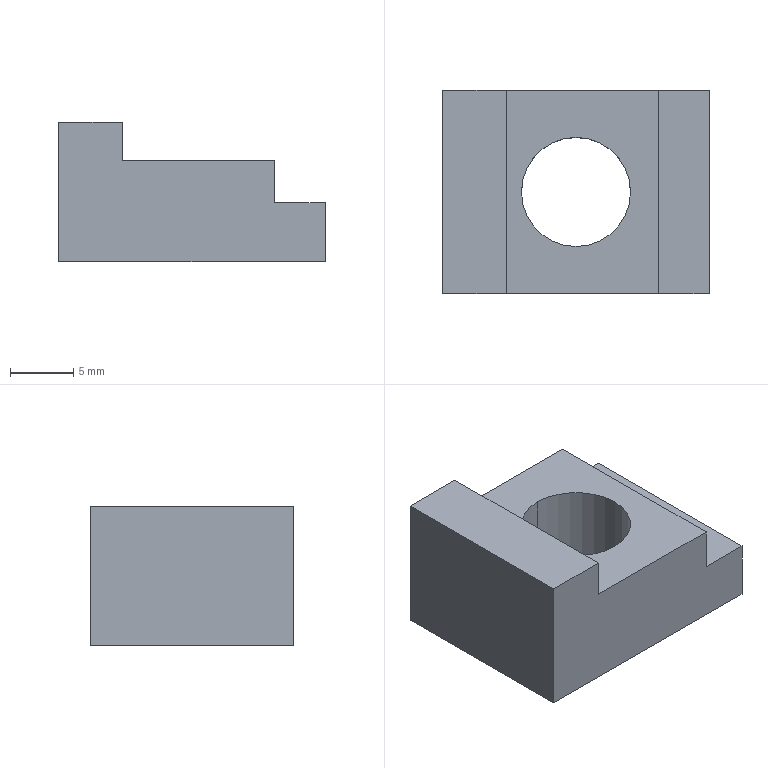Part | STEP file | 1_id1418_x_t | 1 solid | 12 faces | box 21 x 16 x 11 mm | volume 2249 mm3 | plane 10 | cylinder 2 | commonest cylinder face diameters 8.6 x2
STEP:
#1=CARTESIAN_POINT('',(0.,0.,0.));
#2=DIRECTION('',(0.,0.,1.));
#3=DIRECTION('',(1.,0.,0.));
#4=AXIS2_PLACEMENT_3D('',#1,#2,#3);
#5=CARTESIAN_POINT('',(17.925,355.5,90.11));
#6=VERTEX_POINT('',#5);
#7=CARTESIAN_POINT('',(17.925,355.5,79.11));
#8=VERTEX_POINT('',#7);
#9=CARTESIAN_POINT('',(17.925,355.5,90.11));
#10=DIRECTION('',(0.,0.,-1.));
#11=VECTOR('',#10,1.);
#12=LINE('',#9,#11);
#13=CARTESIAN_POINT('',(17.925,355.5,79.11));
#14=DIRECTION('',(1.,0.,0.));
#15=DIRECTION('',(0.,-1.,0.));
#16=AXIS2_PLACEMENT_3D('',#13,#14,#15);
#17=PLANE('',#16);
#18=CARTESIAN_POINT('',(0.,-11.));
#19=DIRECTION('',(0.,1.));
#20=VECTOR('',#19,1.);
#21=LINE('',#18,#20);
#22=(GEOMETRIC_REPRESENTATION_CONTEXT(2)PARAMETRIC_REPRESENTATION_CONTEXT()REPRESENTATION_CONTEXT('',''));
#23=DEFINITIONAL_REPRESENTATION('',(#21),#22);
#24=PCURVE('',#17,#23);
#25=CARTESIAN_POINT('',(38.925,355.5,79.11));
#26=DIRECTION('',(0.,-1.,0.));
#27=DIRECTION('',(0.,0.,1.));
#28=AXIS2_PLACEMENT_3D('',#25,#26,#27);
#29=PLANE('',#28);
#30=CARTESIAN_POINT('',(11.,21.));
#31=DIRECTION('',(-1.,0.));
#32=VECTOR('',#31,1.);
#33=LINE('',#30,#32);
#34=(GEOMETRIC_REPRESENTATION_CONTEXT(2)PARAMETRIC_REPRESENTATION_CONTEXT()REPRESENTATION_CONTEXT('',''));
#35=DEFINITIONAL_REPRESENTATION('',(#33),#34);
#36=PCURVE('',#29,#35);
#37=SURFACE_CURVE('',#12,(#24,#36),.PCURVE_S1.);
#38=EDGE_CURVE('',#6,#8,#37,.T.);
#39=ORIENTED_EDGE('',*,*,#38,.T.);
#40=CARTESIAN_POINT('',(17.925,339.5,79.11));
#41=VERTEX_POINT('',#40);
#42=CARTESIAN_POINT('',(17.925,339.5,79.11));
#43=DIRECTION('',(0.,1.,0.));
#44=VECTOR('',#43,1.);
#45=LINE('',#42,#44);
#46=CARTESIAN_POINT('',(16.,0.));
#47=DIRECTION('',(-1.,0.));
#48=VECTOR('',#47,1.);
#49=LINE('',#46,#48);
#50=(GEOMETRIC_REPRESENTATION_CONTEXT(2)PARAMETRIC_REPRESENTATION_CONTEXT()REPRESENTATION_CONTEXT('',''));
#51=DEFINITIONAL_REPRESENTATION('',(#49),#50);
#52=PCURVE('',#17,#51);
#53=CARTESIAN_POINT('',(38.925,339.5,79.11));
#54=DIRECTION('',(0.,0.,-1.));
#55=DIRECTION('',(-0.5,0.866,0.));
#56=AXIS2_PLACEMENT_3D('',#53,#54,#55);
#57=PLANE('',#56);
#58=CARTESIAN_POINT('',(10.5,-18.187));
#59=DIRECTION('',(0.866,0.5));
#60=VECTOR('',#59,1.);
#61=LINE('',#58,#60);
#62=(GEOMETRIC_REPRESENTATION_CONTEXT(2)PARAMETRIC_REPRESENTATION_CONTEXT()REPRESENTATION_CONTEXT('',''));
#63=DEFINITIONAL_REPRESENTATION('',(#61),#62);
#64=PCURVE('',#57,#63);
#65=SURFACE_CURVE('',#45,(#52,#64),.PCURVE_S1.);
#66=EDGE_CURVE('',#41,#8,#65,.T.);
#67=ORIENTED_EDGE('',*,*,#66,.F.);
#68=CARTESIAN_POINT('',(17.925,339.5,90.11));
#69=VERTEX_POINT('',#68);
#70=CARTESIAN_POINT('',(17.925,339.5,90.11));
#71=DIRECTION('',(0.,0.,-1.));
#72=VECTOR('',#71,1.);
#73=LINE('',#70,#72);
#74=CARTESIAN_POINT('',(16.,-11.));
#75=DIRECTION('',(0.,1.));
#76=VECTOR('',#75,1.);
#77=LINE('',#74,#76);
#78=(GEOMETRIC_REPRESENTATION_CONTEXT(2)PARAMETRIC_REPRESENTATION_CONTEXT()REPRESENTATION_CONTEXT('',''));
#79=DEFINITIONAL_REPRESENTATION('',(#77),#78);
#80=PCURVE('',#17,#79);
#81=CARTESIAN_POINT('',(17.925,339.5,79.11));
#82=DIRECTION('',(0.,1.,0.));
#83=DIRECTION('',(0.,0.,-1.));
#84=AXIS2_PLACEMENT_3D('',#81,#82,#83);
#85=PLANE('',#84);
#86=CARTESIAN_POINT('',(-11.,0.));
#87=DIRECTION('',(1.,0.));
#88=VECTOR('',#87,1.);
#89=LINE('',#86,#88);
#90=(GEOMETRIC_REPRESENTATION_CONTEXT(2)PARAMETRIC_REPRESENTATION_CONTEXT()REPRESENTATION_CONTEXT('',''));
#91=DEFINITIONAL_REPRESENTATION('',(#89),#90);
#92=PCURVE('',#85,#91);
#93=SURFACE_CURVE('',#73,(#80,#92),.PCURVE_S1.);
#94=EDGE_CURVE('',#69,#41,#93,.T.);
#95=ORIENTED_EDGE('',*,*,#94,.F.);
#96=CARTESIAN_POINT('',(17.925,355.5,90.11));
#97=DIRECTION('',(0.,-1.,0.));
#98=VECTOR('',#97,1.);
#99=LINE('',#96,#98);
#100=CARTESIAN_POINT('',(0.,-11.));
#101=DIRECTION('',(1.,0.));
#102=VECTOR('',#101,1.);
#103=LINE('',#100,#102);
#104=(GEOMETRIC_REPRESENTATION_CONTEXT(2)PARAMETRIC_REPRESENTATION_CONTEXT()REPRESENTATION_CONTEXT('',''));
#105=DEFINITIONAL_REPRESENTATION('',(#103),#104);
#106=PCURVE('',#17,#105);
#107=CARTESIAN_POINT('',(22.925,355.5,90.11));
#108=DIRECTION('',(0.,0.,1.));
#109=DIRECTION('',(0.866,0.5,0.));
#110=AXIS2_PLACEMENT_3D('',#107,#108,#109);
#111=PLANE('',#110);
#112=CARTESIAN_POINT('',(-4.33,2.5));
#113=DIRECTION('',(-0.5,-0.866));
#114=VECTOR('',#113,1.);
#115=LINE('',#112,#114);
#116=(GEOMETRIC_REPRESENTATION_CONTEXT(2)PARAMETRIC_REPRESENTATION_CONTEXT()REPRESENTATION_CONTEXT('',''));
#117=DEFINITIONAL_REPRESENTATION('',(#115),#116);
#118=PCURVE('',#111,#117);
#119=SURFACE_CURVE('',#99,(#106,#118),.PCURVE_S1.);
#120=EDGE_CURVE('',#6,#69,#119,.T.);
#121=ORIENTED_EDGE('',*,*,#120,.F.);
#122=EDGE_LOOP('',(#39,#67,#95,#121));
#123=FACE_BOUND('',#122,.T.);
#124=ADVANCED_FACE('',(#123),#17,.F.);
#125=ORIENTED_EDGE('',*,*,#120,.T.);
#126=CARTESIAN_POINT('',(22.925,339.5,90.11));
#127=VERTEX_POINT('',#126);
#128=CARTESIAN_POINT('',(17.925,339.5,90.11));
#129=DIRECTION('',(1.,0.,0.));
#130=VECTOR('',#129,1.);
#131=LINE('',#128,#130);
#132=CARTESIAN_POINT('',(-12.33,-11.356));
#133=DIRECTION('',(0.866,-0.5));
#134=VECTOR('',#133,1.);
#135=LINE('',#132,#134);
#136=(GEOMETRIC_REPRESENTATION_CONTEXT(2)PARAMETRIC_REPRESENTATION_CONTEXT()REPRESENTATION_CONTEXT('',''));
#137=DEFINITIONAL_REPRESENTATION('',(#135),#136);
#138=PCURVE('',#111,#137);
#139=CARTESIAN_POINT('',(-11.,0.));
#140=DIRECTION('',(0.,-1.));
#141=VECTOR('',#140,1.);
#142=LINE('',#139,#141);
#143=(GEOMETRIC_REPRESENTATION_CONTEXT(2)PARAMETRIC_REPRESENTATION_CONTEXT()REPRESENTATION_CONTEXT('',''));
#144=DEFINITIONAL_REPRESENTATION('',(#142),#143);
#145=PCURVE('',#85,#144);
#146=SURFACE_CURVE('',#131,(#138,#145),.PCURVE_S1.);
#147=EDGE_CURVE('',#69,#127,#146,.T.);
#148=ORIENTED_EDGE('',*,*,#147,.T.);
#149=CARTESIAN_POINT('',(22.925,355.5,90.11));
#150=VERTEX_POINT('',#149);
#151=CARTESIAN_POINT('',(22.925,339.5,90.11));
#152=DIRECTION('',(0.,1.,0.));
#153=VECTOR('',#152,1.);
#154=LINE('',#151,#153);
#155=CARTESIAN_POINT('',(-8.,-13.856));
#156=DIRECTION('',(0.5,0.866));
#157=VECTOR('',#156,1.);
#158=LINE('',#155,#157);
#159=(GEOMETRIC_REPRESENTATION_CONTEXT(2)PARAMETRIC_REPRESENTATION_CONTEXT()REPRESENTATION_CONTEXT('',''));
#160=DEFINITIONAL_REPRESENTATION('',(#158),#159);
#161=PCURVE('',#111,#160);
#162=CARTESIAN_POINT('',(22.925,355.5,90.11));
#163=DIRECTION('',(-1.,0.,0.));
#164=DIRECTION('',(0.,0.,1.));
#165=AXIS2_PLACEMENT_3D('',#162,#163,#164);
#166=PLANE('',#165);
#167=CARTESIAN_POINT('',(0.,-16.));
#168=DIRECTION('',(0.,1.));
#169=VECTOR('',#168,1.);
#170=LINE('',#167,#169);
#171=(GEOMETRIC_REPRESENTATION_CONTEXT(2)PARAMETRIC_REPRESENTATION_CONTEXT()REPRESENTATION_CONTEXT('',''));
#172=DEFINITIONAL_REPRESENTATION('',(#170),#171);
#173=PCURVE('',#166,#172);
#174=SURFACE_CURVE('',#154,(#161,#173),.PCURVE_S1.);
#175=EDGE_CURVE('',#127,#150,#174,.T.);
#176=ORIENTED_EDGE('',*,*,#175,.T.);
#177=CARTESIAN_POINT('',(22.925,355.5,90.11));
#178=DIRECTION('',(-1.,0.,0.));
#179=VECTOR('',#178,1.);
#180=LINE('',#177,#179);
#181=CARTESIAN_POINT('',(0.,0.));
#182=DIRECTION('',(-0.866,0.5));
#183=VECTOR('',#182,1.);
#184=LINE('',#181,#183);
#185=(GEOMETRIC_REPRESENTATION_CONTEXT(2)PARAMETRIC_REPRESENTATION_CONTEXT()REPRESENTATION_CONTEXT('',''));
#186=DEFINITIONAL_REPRESENTATION('',(#184),#185);
#187=PCURVE('',#111,#186);
#188=CARTESIAN_POINT('',(11.,16.));
#189=DIRECTION('',(0.,1.));
#190=VECTOR('',#189,1.);
#191=LINE('',#188,#190);
#192=(GEOMETRIC_REPRESENTATION_CONTEXT(2)PARAMETRIC_REPRESENTATION_CONTEXT()REPRESENTATION_CONTEXT('',''));
#193=DEFINITIONAL_REPRESENTATION('',(#191),#192);
#194=PCURVE('',#29,#193);
#195=SURFACE_CURVE('',#180,(#187,#194),.PCURVE_S1.);
#196=EDGE_CURVE('',#150,#6,#195,.T.);
#197=ORIENTED_EDGE('',*,*,#196,.T.);
#198=EDGE_LOOP('',(#125,#148,#176,#197));
#199=FACE_BOUND('',#198,.T.);
#200=ADVANCED_FACE('',(#199),#111,.T.);
#201=CARTESIAN_POINT('',(34.925,355.5,83.76));
#202=VERTEX_POINT('',#201);
#203=CARTESIAN_POINT('',(34.925,355.5,87.11));
#204=VERTEX_POINT('',#203);
#205=CARTESIAN_POINT('',(34.925,355.5,83.76));
#206=DIRECTION('',(0.,0.,1.));
#207=VECTOR('',#206,1.);
#208=LINE('',#205,#207);
#209=CARTESIAN_POINT('',(4.65,4.));
#210=DIRECTION('',(1.,0.));
#211=VECTOR('',#210,1.);
#212=LINE('',#209,#211);
#213=(GEOMETRIC_REPRESENTATION_CONTEXT(2)PARAMETRIC_REPRESENTATION_CONTEXT()REPRESENTATION_CONTEXT('',''));
#214=DEFINITIONAL_REPRESENTATION('',(#212),#213);
#215=PCURVE('',#29,#214);
#216=CARTESIAN_POINT('',(34.925,355.5,87.11));
#217=DIRECTION('',(-1.,0.,0.));
#218=DIRECTION('',(0.,0.,1.));
#219=AXIS2_PLACEMENT_3D('',#216,#217,#218);
#220=PLANE('',#219);
#221=CARTESIAN_POINT('',(-3.35,0.));
#222=DIRECTION('',(1.,0.));
#223=VECTOR('',#222,1.);
#224=LINE('',#221,#223);
#225=(GEOMETRIC_REPRESENTATION_CONTEXT(2)PARAMETRIC_REPRESENTATION_CONTEXT()REPRESENTATION_CONTEXT('',''));
#226=DEFINITIONAL_REPRESENTATION('',(#224),#225);
#227=PCURVE('',#220,#226);
#228=SURFACE_CURVE('',#208,(#215,#227),.PCURVE_S1.);
#229=EDGE_CURVE('',#202,#204,#228,.T.);
#230=ORIENTED_EDGE('',*,*,#229,.F.);
#231=CARTESIAN_POINT('',(38.925,355.5,83.76));
#232=VERTEX_POINT('',#231);
#233=CARTESIAN_POINT('',(38.925,355.5,83.76));
#234=DIRECTION('',(-1.,0.,0.));
#235=VECTOR('',#234,1.);
#236=LINE('',#233,#235);
#237=CARTESIAN_POINT('',(4.65,0.));
#238=DIRECTION('',(0.,1.));
#239=VECTOR('',#238,1.);
#240=LINE('',#237,#239);
#241=(GEOMETRIC_REPRESENTATION_CONTEXT(2)PARAMETRIC_REPRESENTATION_CONTEXT()REPRESENTATION_CONTEXT('',''));
#242=DEFINITIONAL_REPRESENTATION('',(#240),#241);
#243=PCURVE('',#29,#242);
#244=CARTESIAN_POINT('',(38.925,339.5,83.76));
#245=DIRECTION('',(0.,0.,-1.));
#246=DIRECTION('',(-0.5,0.866,0.));
#247=AXIS2_PLACEMENT_3D('',#244,#245,#246);
#248=PLANE('',#247);
#249=CARTESIAN_POINT('',(13.856,8.));
#250=DIRECTION('',(0.5,-0.866));
#251=VECTOR('',#250,1.);
#252=LINE('',#249,#251);
#253=(GEOMETRIC_REPRESENTATION_CONTEXT(2)PARAMETRIC_REPRESENTATION_CONTEXT()REPRESENTATION_CONTEXT('',''));
#254=DEFINITIONAL_REPRESENTATION('',(#252),#253);
#255=PCURVE('',#248,#254);
#256=SURFACE_CURVE('',#236,(#243,#255),.PCURVE_S1.);
#257=EDGE_CURVE('',#232,#202,#256,.T.);
#258=ORIENTED_EDGE('',*,*,#257,.F.);
#259=CARTESIAN_POINT('',(38.925,355.5,79.11));
#260=VERTEX_POINT('',#259);
#261=CARTESIAN_POINT('',(38.925,355.5,83.76));
#262=DIRECTION('',(0.,0.,-1.));
#263=VECTOR('',#262,1.);
#264=LINE('',#261,#263);
#265=CARTESIAN_POINT('',(4.65,0.));
#266=DIRECTION('',(-1.,0.));
#267=VECTOR('',#266,1.);
#268=LINE('',#265,#267);
#269=(GEOMETRIC_REPRESENTATION_CONTEXT(2)PARAMETRIC_REPRESENTATION_CONTEXT()REPRESENTATION_CONTEXT('',''));
#270=DEFINITIONAL_REPRESENTATION('',(#268),#269);
#271=PCURVE('',#29,#270);
#272=CARTESIAN_POINT('',(38.925,339.5,79.11));
#273=DIRECTION('',(-1.,0.,0.));
#274=DIRECTION('',(0.,0.,1.));
#275=AXIS2_PLACEMENT_3D('',#272,#273,#274);
#276=PLANE('',#275);
#277=CARTESIAN_POINT('',(4.65,16.));
#278=DIRECTION('',(-1.,0.));
#279=VECTOR('',#278,1.);
#280=LINE('',#277,#279);
#281=(GEOMETRIC_REPRESENTATION_CONTEXT(2)PARAMETRIC_REPRESENTATION_CONTEXT()REPRESENTATION_CONTEXT('',''));
#282=DEFINITIONAL_REPRESENTATION('',(#280),#281);
#283=PCURVE('',#276,#282);
#284=SURFACE_CURVE('',#264,(#271,#283),.PCURVE_S1.);
#285=EDGE_CURVE('',#232,#260,#284,.T.);
#286=ORIENTED_EDGE('',*,*,#285,.T.);
#287=CARTESIAN_POINT('',(17.925,355.5,79.11));
#288=DIRECTION('',(1.,0.,0.));
#289=VECTOR('',#288,1.);
#290=LINE('',#287,#289);
#291=CARTESIAN_POINT('',(0.,21.));
#292=DIRECTION('',(0.,-1.));
#293=VECTOR('',#292,1.);
#294=LINE('',#291,#293);
#295=(GEOMETRIC_REPRESENTATION_CONTEXT(2)PARAMETRIC_REPRESENTATION_CONTEXT()REPRESENTATION_CONTEXT('',''));
#296=DEFINITIONAL_REPRESENTATION('',(#294),#295);
#297=PCURVE('',#29,#296);
#298=CARTESIAN_POINT('',(24.356,-10.187));
#299=DIRECTION('',(-0.5,0.866));
#300=VECTOR('',#299,1.);
#301=LINE('',#298,#300);
#302=(GEOMETRIC_REPRESENTATION_CONTEXT(2)PARAMETRIC_REPRESENTATION_CONTEXT()REPRESENTATION_CONTEXT('',''));
#303=DEFINITIONAL_REPRESENTATION('',(#301),#302);
#304=PCURVE('',#57,#303);
#305=SURFACE_CURVE('',#290,(#297,#304),.PCURVE_S1.);
#306=EDGE_CURVE('',#8,#260,#305,.T.);
#307=ORIENTED_EDGE('',*,*,#306,.F.);
#308=ORIENTED_EDGE('',*,*,#38,.F.);
#309=ORIENTED_EDGE('',*,*,#196,.F.);
#310=CARTESIAN_POINT('',(22.925,355.5,87.11));
#311=VERTEX_POINT('',#310);
#312=CARTESIAN_POINT('',(22.925,355.5,87.11));
#313=DIRECTION('',(0.,0.,1.));
#314=VECTOR('',#313,1.);
#315=LINE('',#312,#314);
#316=CARTESIAN_POINT('',(8.,16.));
#317=DIRECTION('',(1.,0.));
#318=VECTOR('',#317,1.);
#319=LINE('',#316,#318);
#320=(GEOMETRIC_REPRESENTATION_CONTEXT(2)PARAMETRIC_REPRESENTATION_CONTEXT()REPRESENTATION_CONTEXT('',''));
#321=DEFINITIONAL_REPRESENTATION('',(#319),#320);
#322=PCURVE('',#29,#321);
#323=CARTESIAN_POINT('',(-3.,0.));
#324=DIRECTION('',(1.,0.));
#325=VECTOR('',#324,1.);
#326=LINE('',#323,#325);
#327=(GEOMETRIC_REPRESENTATION_CONTEXT(2)PARAMETRIC_REPRESENTATION_CONTEXT()REPRESENTATION_CONTEXT('',''));
#328=DEFINITIONAL_REPRESENTATION('',(#326),#327);
#329=PCURVE('',#166,#328);
#330=SURFACE_CURVE('',#315,(#322,#329),.PCURVE_S1.);
#331=EDGE_CURVE('',#311,#150,#330,.T.);
#332=ORIENTED_EDGE('',*,*,#331,.F.);
#333=CARTESIAN_POINT('',(34.925,355.5,87.11));
#334=DIRECTION('',(-1.,0.,0.));
#335=VECTOR('',#334,1.);
#336=LINE('',#333,#335);
#337=CARTESIAN_POINT('',(8.,4.));
#338=DIRECTION('',(0.,1.));
#339=VECTOR('',#338,1.);
#340=LINE('',#337,#339);
#341=(GEOMETRIC_REPRESENTATION_CONTEXT(2)PARAMETRIC_REPRESENTATION_CONTEXT()REPRESENTATION_CONTEXT('',''));
#342=DEFINITIONAL_REPRESENTATION('',(#340),#341);
#343=PCURVE('',#29,#342);
#344=CARTESIAN_POINT('',(17.925,339.5,87.11));
#345=DIRECTION('',(0.,0.,1.));
#346=DIRECTION('',(0.866,0.5,0.));
#347=AXIS2_PLACEMENT_3D('',#344,#345,#346);
#348=PLANE('',#347);
#349=CARTESIAN_POINT('',(22.722,5.356));
#350=DIRECTION('',(-0.866,0.5));
#351=VECTOR('',#350,1.);
#352=LINE('',#349,#351);
#353=(GEOMETRIC_REPRESENTATION_CONTEXT(2)PARAMETRIC_REPRESENTATION_CONTEXT()REPRESENTATION_CONTEXT('',''));
#354=DEFINITIONAL_REPRESENTATION('',(#352),#353);
#355=PCURVE('',#348,#354);
#356=SURFACE_CURVE('',#336,(#343,#355),.PCURVE_S1.);
#357=EDGE_CURVE('',#204,#311,#356,.T.);
#358=ORIENTED_EDGE('',*,*,#357,.F.);
#359=EDGE_LOOP('',(#230,#258,#286,#307,#308,#309,#332,#358));
#360=FACE_BOUND('',#359,.T.);
#361=ADVANCED_FACE('',(#360),#29,.F.);
#362=CARTESIAN_POINT('',(34.925,339.5,87.11));
#363=VERTEX_POINT('',#362);
#364=CARTESIAN_POINT('',(34.925,339.5,87.11));
#365=DIRECTION('',(0.,1.,0.));
#366=VECTOR('',#365,1.);
#367=LINE('',#364,#366);
#368=CARTESIAN_POINT('',(14.722,-8.5));
#369=DIRECTION('',(0.5,0.866));
#370=VECTOR('',#369,1.);
#371=LINE('',#368,#370);
#372=(GEOMETRIC_REPRESENTATION_CONTEXT(2)PARAMETRIC_REPRESENTATION_CONTEXT()REPRESENTATION_CONTEXT('',''));
#373=DEFINITIONAL_REPRESENTATION('',(#371),#372);
#374=PCURVE('',#348,#373);
#375=CARTESIAN_POINT('',(0.,-16.));
#376=DIRECTION('',(0.,1.));
#377=VECTOR('',#376,1.);
#378=LINE('',#375,#377);
#379=(GEOMETRIC_REPRESENTATION_CONTEXT(2)PARAMETRIC_REPRESENTATION_CONTEXT()REPRESENTATION_CONTEXT('',''));
#380=DEFINITIONAL_REPRESENTATION('',(#378),#379);
#381=PCURVE('',#220,#380);
#382=SURFACE_CURVE('',#367,(#374,#381),.PCURVE_S1.);
#383=EDGE_CURVE('',#363,#204,#382,.T.);
#384=ORIENTED_EDGE('',*,*,#383,.T.);
#385=ORIENTED_EDGE('',*,*,#357,.T.);
#386=CARTESIAN_POINT('',(22.925,339.5,87.11));
#387=VERTEX_POINT('',#386);
#388=CARTESIAN_POINT('',(22.925,355.5,87.11));
#389=DIRECTION('',(0.,-1.,0.));
#390=VECTOR('',#389,1.);
#391=LINE('',#388,#390);
#392=CARTESIAN_POINT('',(12.33,11.356));
#393=DIRECTION('',(-0.5,-0.866));
#394=VECTOR('',#393,1.);
#395=LINE('',#392,#394);
#396=(GEOMETRIC_REPRESENTATION_CONTEXT(2)PARAMETRIC_REPRESENTATION_CONTEXT()REPRESENTATION_CONTEXT('',''));
#397=DEFINITIONAL_REPRESENTATION('',(#395),#396);
#398=PCURVE('',#348,#397);
#399=CARTESIAN_POINT('',(-3.,0.));
#400=DIRECTION('',(0.,-1.));
#401=VECTOR('',#400,1.);
#402=LINE('',#399,#401);
#403=(GEOMETRIC_REPRESENTATION_CONTEXT(2)PARAMETRIC_REPRESENTATION_CONTEXT()REPRESENTATION_CONTEXT('',''));
#404=DEFINITIONAL_REPRESENTATION('',(#402),#403);
#405=PCURVE('',#166,#404);
#406=SURFACE_CURVE('',#391,(#398,#405),.PCURVE_S1.);
#407=EDGE_CURVE('',#311,#387,#406,.T.);
#408=ORIENTED_EDGE('',*,*,#407,.T.);
#409=CARTESIAN_POINT('',(22.925,339.5,87.11));
#410=DIRECTION('',(1.,0.,0.));
#411=VECTOR('',#410,1.);
#412=LINE('',#409,#411);
#413=CARTESIAN_POINT('',(4.33,-2.5));
#414=DIRECTION('',(0.866,-0.5));
#415=VECTOR('',#414,1.);
#416=LINE('',#413,#415);
#417=(GEOMETRIC_REPRESENTATION_CONTEXT(2)PARAMETRIC_REPRESENTATION_CONTEXT()REPRESENTATION_CONTEXT('',''));
#418=DEFINITIONAL_REPRESENTATION('',(#416),#417);
#419=PCURVE('',#348,#418);
#420=CARTESIAN_POINT('',(-8.,-5.));
#421=DIRECTION('',(0.,-1.));
#422=VECTOR('',#421,1.);
#423=LINE('',#420,#422);
#424=(GEOMETRIC_REPRESENTATION_CONTEXT(2)PARAMETRIC_REPRESENTATION_CONTEXT()REPRESENTATION_CONTEXT('',''));
#425=DEFINITIONAL_REPRESENTATION('',(#423),#424);
#426=PCURVE('',#85,#425);
#427=SURFACE_CURVE('',#412,(#419,#426),.PCURVE_S1.);
#428=EDGE_CURVE('',#387,#363,#427,.T.);
#429=ORIENTED_EDGE('',*,*,#428,.T.);
#430=EDGE_LOOP('',(#384,#385,#408,#429));
#431=FACE_BOUND('',#430,.T.);
#432=CARTESIAN_POINT('',(28.425,351.8,87.11));
#433=VERTEX_POINT('',#432);
#434=CARTESIAN_POINT('',(28.425,343.2,87.11));
#435=VERTEX_POINT('',#434);
#436=CARTESIAN_POINT('',(28.425,347.5,87.11));
#437=DIRECTION('',(0.,0.,-1.));
#438=DIRECTION('',(0.,1.,0.));
#439=AXIS2_PLACEMENT_3D('',#436,#437,#438);
#440=CIRCLE('',#439,4.3);
#441=CARTESIAN_POINT('',(15.243,5.402));
#442=CARTESIAN_POINT('',(21.693,1.678));
#443=CARTESIAN_POINT('',(15.243,-2.046));
#444=CARTESIAN_POINT('',(8.793,-5.77));
#445=CARTESIAN_POINT('',(8.793,1.678));
#446=CARTESIAN_POINT('',(8.793,9.126));
#447=CARTESIAN_POINT('',(15.243,5.402));
#448=(BOUNDED_CURVE()B_SPLINE_CURVE(2,(#441,#442,#443,#444,#445,#446,#447),.UNSPECIFIED.,.T.,.F.)B_SPLINE_CURVE_WITH_KNOTS((1,2,2,2,2,1),(-2.094,0.,2.094,4.189,6.283,8.378),.UNSPECIFIED.)CURVE()GEOMETRIC_REPRESENTATION_ITEM()RATIONAL_B_SPLINE_CURVE((1.,0.5,1.,0.5,1.,0.5,1.))REPRESENTATION_ITEM(''));
#449=(GEOMETRIC_REPRESENTATION_CONTEXT(2)PARAMETRIC_REPRESENTATION_CONTEXT()REPRESENTATION_CONTEXT('',''));
#450=DEFINITIONAL_REPRESENTATION('',(#448),#449);
#451=PCURVE('',#348,#450);
#452=CARTESIAN_POINT('',(28.425,347.5,107.03));
#453=DIRECTION('',(0.,0.,1.));
#454=DIRECTION('',(0.,1.,0.));
#455=AXIS2_PLACEMENT_3D('',#452,#453,#454);
#456=CYLINDRICAL_SURFACE('',#455,4.3);
#457=CARTESIAN_POINT('',(6.283,-19.92));
#458=DIRECTION('',(-1.,0.));
#459=VECTOR('',#458,1.);
#460=LINE('',#457,#459);
#461=(GEOMETRIC_REPRESENTATION_CONTEXT(2)PARAMETRIC_REPRESENTATION_CONTEXT()REPRESENTATION_CONTEXT('',''));
#462=DEFINITIONAL_REPRESENTATION('',(#460),#461);
#463=PCURVE('',#456,#462);
#464=SURFACE_CURVE('',#440,(#451,#463),.PCURVE_S1.);
#465=EDGE_CURVE('',#433,#435,#464,.T.);
#466=ORIENTED_EDGE('',*,*,#465,.T.);
#467=CARTESIAN_POINT('',(24.125,347.5,87.11));
#468=VERTEX_POINT('',#467);
#469=CARTESIAN_POINT('',(28.425,347.5,87.11));
#470=DIRECTION('',(0.,0.,-1.));
#471=DIRECTION('',(0.,-1.,0.));
#472=AXIS2_PLACEMENT_3D('',#469,#470,#471);
#473=CIRCLE('',#472,4.3);
#474=CARTESIAN_POINT('',(10.943,-2.046));
#475=CARTESIAN_POINT('',(4.493,1.678));
#476=CARTESIAN_POINT('',(10.943,5.402));
#477=CARTESIAN_POINT('',(17.393,9.126));
#478=CARTESIAN_POINT('',(17.393,1.678));
#479=CARTESIAN_POINT('',(17.393,-5.77));
#480=CARTESIAN_POINT('',(10.943,-2.046));
#481=(BOUNDED_CURVE()B_SPLINE_CURVE(2,(#474,#475,#476,#477,#478,#479,#480),.UNSPECIFIED.,.T.,.F.)B_SPLINE_CURVE_WITH_KNOTS((1,2,2,2,2,1),(-2.094,0.,2.094,4.189,6.283,8.378),.UNSPECIFIED.)CURVE()GEOMETRIC_REPRESENTATION_ITEM()RATIONAL_B_SPLINE_CURVE((1.,0.5,1.,0.5,1.,0.5,1.))REPRESENTATION_ITEM(''));
#482=(GEOMETRIC_REPRESENTATION_CONTEXT(2)PARAMETRIC_REPRESENTATION_CONTEXT()REPRESENTATION_CONTEXT('',''));
#483=DEFINITIONAL_REPRESENTATION('',(#481),#482);
#484=PCURVE('',#348,#483);
#485=CARTESIAN_POINT('',(28.425,347.5,107.03));
#486=DIRECTION('',(0.,0.,1.));
#487=DIRECTION('',(0.,1.,0.));
#488=AXIS2_PLACEMENT_3D('',#485,#486,#487);
#489=CYLINDRICAL_SURFACE('',#488,4.3);
#490=CARTESIAN_POINT('',(3.142,-19.92));
#491=DIRECTION('',(-1.,0.));
#492=VECTOR('',#491,1.);
#493=LINE('',#490,#492);
#494=(GEOMETRIC_REPRESENTATION_CONTEXT(2)PARAMETRIC_REPRESENTATION_CONTEXT()REPRESENTATION_CONTEXT('',''));
#495=DEFINITIONAL_REPRESENTATION('',(#493),#494);
#496=PCURVE('',#489,#495);
#497=SURFACE_CURVE('',#473,(#484,#496),.PCURVE_S1.);
#498=EDGE_CURVE('',#435,#468,#497,.T.);
#499=ORIENTED_EDGE('',*,*,#498,.T.);
#500=CARTESIAN_POINT('',(28.425,347.5,87.11));
#501=DIRECTION('',(0.,0.,-1.));
#502=DIRECTION('',(-1.,0.,0.));
#503=AXIS2_PLACEMENT_3D('',#500,#501,#502);
#504=CIRCLE('',#503,4.3);
#505=CARTESIAN_POINT('',(9.369,3.828));
#506=CARTESIAN_POINT('',(13.093,10.278));
#507=CARTESIAN_POINT('',(16.817,3.828));
#508=CARTESIAN_POINT('',(20.541,-2.622));
#509=CARTESIAN_POINT('',(13.093,-2.622));
#510=CARTESIAN_POINT('',(5.645,-2.622));
#511=CARTESIAN_POINT('',(9.369,3.828));
#512=(BOUNDED_CURVE()B_SPLINE_CURVE(2,(#505,#506,#507,#508,#509,#510,#511),.UNSPECIFIED.,.T.,.F.)B_SPLINE_CURVE_WITH_KNOTS((1,2,2,2,2,1),(-2.094,0.,2.094,4.189,6.283,8.378),.UNSPECIFIED.)CURVE()GEOMETRIC_REPRESENTATION_ITEM()RATIONAL_B_SPLINE_CURVE((1.,0.5,1.,0.5,1.,0.5,1.))REPRESENTATION_ITEM(''));
#513=(GEOMETRIC_REPRESENTATION_CONTEXT(2)PARAMETRIC_REPRESENTATION_CONTEXT()REPRESENTATION_CONTEXT('',''));
#514=DEFINITIONAL_REPRESENTATION('',(#512),#513);
#515=PCURVE('',#348,#514);
#516=CARTESIAN_POINT('',(1.571,-19.92));
#517=DIRECTION('',(-1.,0.));
#518=VECTOR('',#517,1.);
#519=LINE('',#516,#518);
#520=(GEOMETRIC_REPRESENTATION_CONTEXT(2)PARAMETRIC_REPRESENTATION_CONTEXT()REPRESENTATION_CONTEXT('',''));
#521=DEFINITIONAL_REPRESENTATION('',(#519),#520);
#522=PCURVE('',#489,#521);
#523=SURFACE_CURVE('',#504,(#515,#522),.PCURVE_S1.);
#524=EDGE_CURVE('',#468,#433,#523,.T.);
#525=ORIENTED_EDGE('',*,*,#524,.T.);
#526=EDGE_LOOP('',(#466,#499,#525));
#527=FACE_BOUND('',#526,.T.);
#528=ADVANCED_FACE('',(#431,#527),#348,.T.);
#529=CARTESIAN_POINT('',(38.925,339.5,79.11));
#530=VERTEX_POINT('',#529);
#531=CARTESIAN_POINT('',(38.925,339.5,79.11));
#532=DIRECTION('',(-1.,0.,0.));
#533=VECTOR('',#532,1.);
#534=LINE('',#531,#533);
#535=CARTESIAN_POINT('',(0.,-21.));
#536=DIRECTION('',(0.,1.));
#537=VECTOR('',#536,1.);
#538=LINE('',#535,#537);
#539=(GEOMETRIC_REPRESENTATION_CONTEXT(2)PARAMETRIC_REPRESENTATION_CONTEXT()REPRESENTATION_CONTEXT('',''));
#540=DEFINITIONAL_REPRESENTATION('',(#538),#539);
#541=PCURVE('',#85,#540);
#542=CARTESIAN_POINT('',(0.,0.));
#543=DIRECTION('',(0.5,-0.866));
#544=VECTOR('',#543,1.);
#545=LINE('',#542,#544);
#546=(GEOMETRIC_REPRESENTATION_CONTEXT(2)PARAMETRIC_REPRESENTATION_CONTEXT()REPRESENTATION_CONTEXT('',''));
#547=DEFINITIONAL_REPRESENTATION('',(#545),#546);
#548=PCURVE('',#57,#547);
#549=SURFACE_CURVE('',#534,(#541,#548),.PCURVE_S1.);
#550=EDGE_CURVE('',#530,#41,#549,.T.);
#551=ORIENTED_EDGE('',*,*,#550,.F.);
#552=CARTESIAN_POINT('',(38.925,339.5,83.76));
#553=VERTEX_POINT('',#552);
#554=CARTESIAN_POINT('',(38.925,339.5,83.76));
#555=DIRECTION('',(0.,0.,-1.));
#556=VECTOR('',#555,1.);
#557=LINE('',#554,#556);
#558=CARTESIAN_POINT('',(-4.65,-21.));
#559=DIRECTION('',(1.,0.));
#560=VECTOR('',#559,1.);
#561=LINE('',#558,#560);
#562=(GEOMETRIC_REPRESENTATION_CONTEXT(2)PARAMETRIC_REPRESENTATION_CONTEXT()REPRESENTATION_CONTEXT('',''));
#563=DEFINITIONAL_REPRESENTATION('',(#561),#562);
#564=PCURVE('',#85,#563);
#565=CARTESIAN_POINT('',(4.65,0.));
#566=DIRECTION('',(-1.,0.));
#567=VECTOR('',#566,1.);
#568=LINE('',#565,#567);
#569=(GEOMETRIC_REPRESENTATION_CONTEXT(2)PARAMETRIC_REPRESENTATION_CONTEXT()REPRESENTATION_CONTEXT('',''));
#570=DEFINITIONAL_REPRESENTATION('',(#568),#569);
#571=PCURVE('',#276,#570);
#572=SURFACE_CURVE('',#557,(#564,#571),.PCURVE_S1.);
#573=EDGE_CURVE('',#553,#530,#572,.T.);
#574=ORIENTED_EDGE('',*,*,#573,.F.);
#575=CARTESIAN_POINT('',(34.925,339.5,83.76));
#576=VERTEX_POINT('',#575);
#577=CARTESIAN_POINT('',(34.925,339.5,83.76));
#578=DIRECTION('',(1.,0.,0.));
#579=VECTOR('',#578,1.);
#580=LINE('',#577,#579);
#581=CARTESIAN_POINT('',(-4.65,-17.));
#582=DIRECTION('',(0.,-1.));
#583=VECTOR('',#582,1.);
#584=LINE('',#581,#583);
#585=(GEOMETRIC_REPRESENTATION_CONTEXT(2)PARAMETRIC_REPRESENTATION_CONTEXT()REPRESENTATION_CONTEXT('',''));
#586=DEFINITIONAL_REPRESENTATION('',(#584),#585);
#587=PCURVE('',#85,#586);
#588=CARTESIAN_POINT('',(2.,-3.464));
#589=DIRECTION('',(-0.5,0.866));
#590=VECTOR('',#589,1.);
#591=LINE('',#588,#590);
#592=(GEOMETRIC_REPRESENTATION_CONTEXT(2)PARAMETRIC_REPRESENTATION_CONTEXT()REPRESENTATION_CONTEXT('',''));
#593=DEFINITIONAL_REPRESENTATION('',(#591),#592);
#594=PCURVE('',#248,#593);
#595=SURFACE_CURVE('',#580,(#587,#594),.PCURVE_S1.);
#596=EDGE_CURVE('',#576,#553,#595,.T.);
#597=ORIENTED_EDGE('',*,*,#596,.F.);
#598=CARTESIAN_POINT('',(34.925,339.5,83.76));
#599=DIRECTION('',(0.,0.,1.));
#600=VECTOR('',#599,1.);
#601=LINE('',#598,#600);
#602=CARTESIAN_POINT('',(-4.65,-17.));
#603=DIRECTION('',(-1.,0.));
#604=VECTOR('',#603,1.);
#605=LINE('',#602,#604);
#606=(GEOMETRIC_REPRESENTATION_CONTEXT(2)PARAMETRIC_REPRESENTATION_CONTEXT()REPRESENTATION_CONTEXT('',''));
#607=DEFINITIONAL_REPRESENTATION('',(#605),#606);
#608=PCURVE('',#85,#607);
#609=CARTESIAN_POINT('',(-3.35,-16.));
#610=DIRECTION('',(1.,0.));
#611=VECTOR('',#610,1.);
#612=LINE('',#609,#611);
#613=(GEOMETRIC_REPRESENTATION_CONTEXT(2)PARAMETRIC_REPRESENTATION_CONTEXT()REPRESENTATION_CONTEXT('',''));
#614=DEFINITIONAL_REPRESENTATION('',(#612),#613);
#615=PCURVE('',#220,#614);
#616=SURFACE_CURVE('',#601,(#608,#615),.PCURVE_S1.);
#617=EDGE_CURVE('',#576,#363,#616,.T.);
#618=ORIENTED_EDGE('',*,*,#617,.T.);
#619=ORIENTED_EDGE('',*,*,#428,.F.);
#620=CARTESIAN_POINT('',(22.925,339.5,87.11));
#621=DIRECTION('',(0.,0.,1.));
#622=VECTOR('',#621,1.);
#623=LINE('',#620,#622);
#624=CARTESIAN_POINT('',(-8.,-5.));
#625=DIRECTION('',(-1.,0.));
#626=VECTOR('',#625,1.);
#627=LINE('',#624,#626);
#628=(GEOMETRIC_REPRESENTATION_CONTEXT(2)PARAMETRIC_REPRESENTATION_CONTEXT()REPRESENTATION_CONTEXT('',''));
#629=DEFINITIONAL_REPRESENTATION('',(#627),#628);
#630=PCURVE('',#85,#629);
#631=CARTESIAN_POINT('',(-3.,-16.));
#632=DIRECTION('',(1.,0.));
#633=VECTOR('',#632,1.);
#634=LINE('',#631,#633);
#635=(GEOMETRIC_REPRESENTATION_CONTEXT(2)PARAMETRIC_REPRESENTATION_CONTEXT()REPRESENTATION_CONTEXT('',''));
#636=DEFINITIONAL_REPRESENTATION('',(#634),#635);
#637=PCURVE('',#166,#636);
#638=SURFACE_CURVE('',#623,(#630,#637),.PCURVE_S1.);
#639=EDGE_CURVE('',#387,#127,#638,.T.);
#640=ORIENTED_EDGE('',*,*,#639,.T.);
#641=ORIENTED_EDGE('',*,*,#147,.F.);
#642=ORIENTED_EDGE('',*,*,#94,.T.);
#643=EDGE_LOOP('',(#551,#574,#597,#618,#619,#640,#641,#642));
#644=FACE_BOUND('',#643,.T.);
#645=ADVANCED_FACE('',(#644),#85,.F.);
#646=ORIENTED_EDGE('',*,*,#331,.T.);
#647=ORIENTED_EDGE('',*,*,#175,.F.);
#648=ORIENTED_EDGE('',*,*,#639,.F.);
#649=ORIENTED_EDGE('',*,*,#407,.F.);
#650=EDGE_LOOP('',(#646,#647,#648,#649));
#651=FACE_BOUND('',#650,.T.);
#652=ADVANCED_FACE('',(#651),#166,.F.);
#653=ORIENTED_EDGE('',*,*,#229,.T.);
#654=ORIENTED_EDGE('',*,*,#383,.F.);
#655=ORIENTED_EDGE('',*,*,#617,.F.);
#656=CARTESIAN_POINT('',(34.925,355.5,83.76));
#657=DIRECTION('',(0.,-1.,0.));
#658=VECTOR('',#657,1.);
#659=LINE('',#656,#658);
#660=CARTESIAN_POINT('',(-3.35,0.));
#661=DIRECTION('',(0.,-1.));
#662=VECTOR('',#661,1.);
#663=LINE('',#660,#662);
#664=(GEOMETRIC_REPRESENTATION_CONTEXT(2)PARAMETRIC_REPRESENTATION_CONTEXT()REPRESENTATION_CONTEXT('',''));
#665=DEFINITIONAL_REPRESENTATION('',(#663),#664);
#666=PCURVE('',#220,#665);
#667=CARTESIAN_POINT('',(15.856,4.536));
#668=DIRECTION('',(-0.866,-0.5));
#669=VECTOR('',#668,1.);
#670=LINE('',#667,#669);
#671=(GEOMETRIC_REPRESENTATION_CONTEXT(2)PARAMETRIC_REPRESENTATION_CONTEXT()REPRESENTATION_CONTEXT('',''));
#672=DEFINITIONAL_REPRESENTATION('',(#670),#671);
#673=PCURVE('',#248,#672);
#674=SURFACE_CURVE('',#659,(#666,#673),.PCURVE_S1.);
#675=EDGE_CURVE('',#202,#576,#674,.T.);
#676=ORIENTED_EDGE('',*,*,#675,.F.);
#677=EDGE_LOOP('',(#653,#654,#655,#676));
#678=FACE_BOUND('',#677,.T.);
#679=ADVANCED_FACE('',(#678),#220,.F.);
#680=ORIENTED_EDGE('',*,*,#596,.T.);
#681=CARTESIAN_POINT('',(38.925,339.5,83.76));
#682=DIRECTION('',(0.,1.,0.));
#683=VECTOR('',#682,1.);
#684=LINE('',#681,#683);
#685=CARTESIAN_POINT('',(0.,0.));
#686=DIRECTION('',(0.866,0.5));
#687=VECTOR('',#686,1.);
#688=LINE('',#685,#687);
#689=(GEOMETRIC_REPRESENTATION_CONTEXT(2)PARAMETRIC_REPRESENTATION_CONTEXT()REPRESENTATION_CONTEXT('',''));
#690=DEFINITIONAL_REPRESENTATION('',(#688),#689);
#691=PCURVE('',#248,#690);
#692=CARTESIAN_POINT('',(4.65,0.));
#693=DIRECTION('',(0.,1.));
#694=VECTOR('',#693,1.);
#695=LINE('',#692,#694);
#696=(GEOMETRIC_REPRESENTATION_CONTEXT(2)PARAMETRIC_REPRESENTATION_CONTEXT()REPRESENTATION_CONTEXT('',''));
#697=DEFINITIONAL_REPRESENTATION('',(#695),#696);
#698=PCURVE('',#276,#697);
#699=SURFACE_CURVE('',#684,(#691,#698),.PCURVE_S1.);
#700=EDGE_CURVE('',#553,#232,#699,.T.);
#701=ORIENTED_EDGE('',*,*,#700,.T.);
#702=ORIENTED_EDGE('',*,*,#257,.T.);
#703=ORIENTED_EDGE('',*,*,#675,.T.);
#704=EDGE_LOOP('',(#680,#701,#702,#703));
#705=FACE_BOUND('',#704,.T.);
#706=ADVANCED_FACE('',(#705),#248,.F.);
#707=ORIENTED_EDGE('',*,*,#573,.T.);
#708=CARTESIAN_POINT('',(38.925,355.5,79.11));
#709=DIRECTION('',(0.,-1.,0.));
#710=VECTOR('',#709,1.);
#711=LINE('',#708,#710);
#712=CARTESIAN_POINT('',(0.,16.));
#713=DIRECTION('',(0.,-1.));
#714=VECTOR('',#713,1.);
#715=LINE('',#712,#714);
#716=(GEOMETRIC_REPRESENTATION_CONTEXT(2)PARAMETRIC_REPRESENTATION_CONTEXT()REPRESENTATION_CONTEXT('',''));
#717=DEFINITIONAL_REPRESENTATION('',(#715),#716);
#718=PCURVE('',#276,#717);
#719=CARTESIAN_POINT('',(13.856,8.));
#720=DIRECTION('',(-0.866,-0.5));
#721=VECTOR('',#720,1.);
#722=LINE('',#719,#721);
#723=(GEOMETRIC_REPRESENTATION_CONTEXT(2)PARAMETRIC_REPRESENTATION_CONTEXT()REPRESENTATION_CONTEXT('',''));
#724=DEFINITIONAL_REPRESENTATION('',(#722),#723);
#725=PCURVE('',#57,#724);
#726=SURFACE_CURVE('',#711,(#718,#725),.PCURVE_S1.);
#727=EDGE_CURVE('',#260,#530,#726,.T.);
#728=ORIENTED_EDGE('',*,*,#727,.F.);
#729=ORIENTED_EDGE('',*,*,#285,.F.);
#730=ORIENTED_EDGE('',*,*,#700,.F.);
#731=EDGE_LOOP('',(#707,#728,#729,#730));
#732=FACE_BOUND('',#731,.T.);
#733=ADVANCED_FACE('',(#732),#276,.F.);
#734=ORIENTED_EDGE('',*,*,#66,.T.);
#735=ORIENTED_EDGE('',*,*,#306,.T.);
#736=ORIENTED_EDGE('',*,*,#727,.T.);
#737=ORIENTED_EDGE('',*,*,#550,.T.);
#738=EDGE_LOOP('',(#734,#735,#736,#737));
#739=FACE_BOUND('',#738,.T.);
#740=CARTESIAN_POINT('',(28.425,351.8,79.11));
#741=VERTEX_POINT('',#740);
#742=CARTESIAN_POINT('',(28.425,343.2,79.11));
#743=VERTEX_POINT('',#742);
#744=CARTESIAN_POINT('',(28.425,347.5,79.11));
#745=DIRECTION('',(0.,0.,1.));
#746=DIRECTION('',(0.,1.,0.));
#747=AXIS2_PLACEMENT_3D('',#744,#745,#746);
#748=CIRCLE('',#747,4.3);
#749=CARTESIAN_POINT('',(15.902,-2.943));
#750=CARTESIAN_POINT('',(19.626,-9.393));
#751=CARTESIAN_POINT('',(12.178,-9.393));
#752=CARTESIAN_POINT('',(4.73,-9.393));
#753=CARTESIAN_POINT('',(8.454,-2.943));
#754=CARTESIAN_POINT('',(12.178,3.507));
#755=CARTESIAN_POINT('',(15.902,-2.943));
#756=(BOUNDED_CURVE()B_SPLINE_CURVE(2,(#749,#750,#751,#752,#753,#754,#755),.UNSPECIFIED.,.T.,.F.)B_SPLINE_CURVE_WITH_KNOTS((1,2,2,2,2,1),(-2.094,0.,2.094,4.189,6.283,8.378),.UNSPECIFIED.)CURVE()GEOMETRIC_REPRESENTATION_ITEM()RATIONAL_B_SPLINE_CURVE((1.,0.5,1.,0.5,1.,0.5,1.))REPRESENTATION_ITEM(''));
#757=(GEOMETRIC_REPRESENTATION_CONTEXT(2)PARAMETRIC_REPRESENTATION_CONTEXT()REPRESENTATION_CONTEXT('',''));
#758=DEFINITIONAL_REPRESENTATION('',(#756),#757);
#759=PCURVE('',#57,#758);
#760=CARTESIAN_POINT('',(0.,-27.92));
#761=DIRECTION('',(1.,0.));
#762=VECTOR('',#761,1.);
#763=LINE('',#760,#762);
#764=(GEOMETRIC_REPRESENTATION_CONTEXT(2)PARAMETRIC_REPRESENTATION_CONTEXT()REPRESENTATION_CONTEXT('',''));
#765=DEFINITIONAL_REPRESENTATION('',(#763),#764);
#766=PCURVE('',#489,#765);
#767=SURFACE_CURVE('',#748,(#759,#766),.PCURVE_S1.);
#768=EDGE_CURVE('',#741,#743,#767,.T.);
#769=ORIENTED_EDGE('',*,*,#768,.T.);
#770=CARTESIAN_POINT('',(32.725,347.5,79.11));
#771=VERTEX_POINT('',#770);
#772=CARTESIAN_POINT('',(28.425,347.5,79.11));
#773=DIRECTION('',(0.,0.,1.));
#774=DIRECTION('',(0.,-1.,0.));
#775=AXIS2_PLACEMENT_3D('',#772,#773,#774);
#776=CIRCLE('',#775,4.3);
#777=CARTESIAN_POINT('',(8.454,-7.243));
#778=CARTESIAN_POINT('',(4.73,-0.7933));
#779=CARTESIAN_POINT('',(12.178,-0.7933));
#780=CARTESIAN_POINT('',(19.626,-0.7933));
#781=CARTESIAN_POINT('',(15.902,-7.243));
#782=CARTESIAN_POINT('',(12.178,-13.693));
#783=CARTESIAN_POINT('',(8.454,-7.243));
#784=(BOUNDED_CURVE()B_SPLINE_CURVE(2,(#777,#778,#779,#780,#781,#782,#783),.UNSPECIFIED.,.T.,.F.)B_SPLINE_CURVE_WITH_KNOTS((1,2,2,2,2,1),(-2.094,0.,2.094,4.189,6.283,8.378),.UNSPECIFIED.)CURVE()GEOMETRIC_REPRESENTATION_ITEM()RATIONAL_B_SPLINE_CURVE((1.,0.5,1.,0.5,1.,0.5,1.))REPRESENTATION_ITEM(''));
#785=(GEOMETRIC_REPRESENTATION_CONTEXT(2)PARAMETRIC_REPRESENTATION_CONTEXT()REPRESENTATION_CONTEXT('',''));
#786=DEFINITIONAL_REPRESENTATION('',(#784),#785);
#787=PCURVE('',#57,#786);
#788=CARTESIAN_POINT('',(3.142,-27.92));
#789=DIRECTION('',(1.,0.));
#790=VECTOR('',#789,1.);
#791=LINE('',#788,#790);
#792=(GEOMETRIC_REPRESENTATION_CONTEXT(2)PARAMETRIC_REPRESENTATION_CONTEXT()REPRESENTATION_CONTEXT('',''));
#793=DEFINITIONAL_REPRESENTATION('',(#791),#792);
#794=PCURVE('',#456,#793);
#795=SURFACE_CURVE('',#776,(#787,#794),.PCURVE_S1.);
#796=EDGE_CURVE('',#743,#771,#795,.T.);
#797=ORIENTED_EDGE('',*,*,#796,.T.);
#798=CARTESIAN_POINT('',(28.425,347.5,79.11));
#799=DIRECTION('',(0.,0.,1.));
#800=DIRECTION('',(1.,0.,0.));
#801=AXIS2_PLACEMENT_3D('',#798,#799,#800);
#802=CIRCLE('',#801,4.3);
#803=CARTESIAN_POINT('',(10.028,-1.369));
#804=CARTESIAN_POINT('',(16.478,2.355));
#805=CARTESIAN_POINT('',(16.478,-5.093));
#806=CARTESIAN_POINT('',(16.478,-12.541));
#807=CARTESIAN_POINT('',(10.028,-8.817));
#808=CARTESIAN_POINT('',(3.578,-5.093));
#809=CARTESIAN_POINT('',(10.028,-1.369));
#810=(BOUNDED_CURVE()B_SPLINE_CURVE(2,(#803,#804,#805,#806,#807,#808,#809),.UNSPECIFIED.,.T.,.F.)B_SPLINE_CURVE_WITH_KNOTS((1,2,2,2,2,1),(-2.094,0.,2.094,4.189,6.283,8.378),.UNSPECIFIED.)CURVE()GEOMETRIC_REPRESENTATION_ITEM()RATIONAL_B_SPLINE_CURVE((1.,0.5,1.,0.5,1.,0.5,1.))REPRESENTATION_ITEM(''));
#811=(GEOMETRIC_REPRESENTATION_CONTEXT(2)PARAMETRIC_REPRESENTATION_CONTEXT()REPRESENTATION_CONTEXT('',''));
#812=DEFINITIONAL_REPRESENTATION('',(#810),#811);
#813=PCURVE('',#57,#812);
#814=CARTESIAN_POINT('',(4.712,-27.92));
#815=DIRECTION('',(1.,0.));
#816=VECTOR('',#815,1.);
#817=LINE('',#814,#816);
#818=(GEOMETRIC_REPRESENTATION_CONTEXT(2)PARAMETRIC_REPRESENTATION_CONTEXT()REPRESENTATION_CONTEXT('',''));
#819=DEFINITIONAL_REPRESENTATION('',(#817),#818);
#820=PCURVE('',#456,#819);
#821=SURFACE_CURVE('',#802,(#813,#820),.PCURVE_S1.);
#822=EDGE_CURVE('',#771,#741,#821,.T.);
#823=ORIENTED_EDGE('',*,*,#822,.T.);
#824=EDGE_LOOP('',(#769,#797,#823));
#825=FACE_BOUND('',#824,.T.);
#826=ADVANCED_FACE('',(#739,#825),#57,.T.);
#827=ORIENTED_EDGE('',*,*,#796,.T.);
#828=ORIENTED_EDGE('',*,*,#822,.T.);
#829=CARTESIAN_POINT('',(28.425,351.8,79.11));
#830=DIRECTION('',(0.,0.,-1.));
#831=VECTOR('',#830,1.);
#832=LINE('',#829,#831);
#833=CARTESIAN_POINT('',(6.283,-27.92));
#834=DIRECTION('',(0.,-1.));
#835=VECTOR('',#834,1.);
#836=LINE('',#833,#835);
#837=(GEOMETRIC_REPRESENTATION_CONTEXT(2)PARAMETRIC_REPRESENTATION_CONTEXT()REPRESENTATION_CONTEXT('',''));
#838=DEFINITIONAL_REPRESENTATION('',(#836),#837);
#839=PCURVE('',#456,#838);
#840=CARTESIAN_POINT('',(0.,-27.92));
#841=DIRECTION('',(0.,-1.));
#842=VECTOR('',#841,1.);
#843=LINE('',#840,#842);
#844=(GEOMETRIC_REPRESENTATION_CONTEXT(2)PARAMETRIC_REPRESENTATION_CONTEXT()REPRESENTATION_CONTEXT('',''));
#845=DEFINITIONAL_REPRESENTATION('',(#843),#844);
#846=PCURVE('',#489,#845);
#847=SURFACE_CURVE('',#832,(#839,#846),.PCURVE_S1.);
#848=EDGE_CURVE('',#433,#741,#847,.T.);
#849=ORIENTED_EDGE('',*,*,#848,.F.);
#850=ORIENTED_EDGE('',*,*,#465,.T.);
#851=CARTESIAN_POINT('',(28.425,343.2,79.11));
#852=DIRECTION('',(0.,0.,1.));
#853=VECTOR('',#852,1.);
#854=LINE('',#851,#853);
#855=CARTESIAN_POINT('',(3.142,-27.92));
#856=DIRECTION('',(0.,1.));
#857=VECTOR('',#856,1.);
#858=LINE('',#855,#857);
#859=(GEOMETRIC_REPRESENTATION_CONTEXT(2)PARAMETRIC_REPRESENTATION_CONTEXT()REPRESENTATION_CONTEXT('',''));
#860=DEFINITIONAL_REPRESENTATION('',(#858),#859);
#861=PCURVE('',#456,#860);
#862=CARTESIAN_POINT('',(3.142,-27.92));
#863=DIRECTION('',(0.,1.));
#864=VECTOR('',#863,1.);
#865=LINE('',#862,#864);
#866=(GEOMETRIC_REPRESENTATION_CONTEXT(2)PARAMETRIC_REPRESENTATION_CONTEXT()REPRESENTATION_CONTEXT('',''));
#867=DEFINITIONAL_REPRESENTATION('',(#865),#866);
#868=PCURVE('',#489,#867);
#869=SURFACE_CURVE('',#854,(#861,#868),.PCURVE_S1.);
#870=EDGE_CURVE('',#743,#435,#869,.T.);
#871=ORIENTED_EDGE('',*,*,#870,.F.);
#872=EDGE_LOOP('',(#827,#828,#849,#850,#871));
#873=FACE_BOUND('',#872,.F.);
#874=ADVANCED_FACE('',(#873),#456,.F.);
#875=ORIENTED_EDGE('',*,*,#768,.T.);
#876=ORIENTED_EDGE('',*,*,#870,.T.);
#877=ORIENTED_EDGE('',*,*,#498,.T.);
#878=ORIENTED_EDGE('',*,*,#524,.T.);
#879=ORIENTED_EDGE('',*,*,#848,.T.);
#880=EDGE_LOOP('',(#875,#876,#877,#878,#879));
#881=FACE_BOUND('',#880,.F.);
#882=ADVANCED_FACE('',(#881),#489,.F.);
#883=CLOSED_SHELL('',(#124,#200,#361,#528,#645,#652,#679,#706,#733,#826,#874,#882));
#884=MANIFOLD_SOLID_BREP('',#883);
#885=(LENGTH_UNIT()NAMED_UNIT(*)SI_UNIT(.MILLI.,.METRE.));
#886=UNCERTAINTY_MEASURE_WITH_UNIT(LENGTH_MEASURE(0.0000001),#885,'','');
#887=(NAMED_UNIT(*)PLANE_ANGLE_UNIT()SI_UNIT($,.RADIAN.));
#888=(NAMED_UNIT(*)SI_UNIT($,.STERADIAN.)SOLID_ANGLE_UNIT());
#889=(GEOMETRIC_REPRESENTATION_CONTEXT(3)GLOBAL_UNCERTAINTY_ASSIGNED_CONTEXT((#886))GLOBAL_UNIT_ASSIGNED_CONTEXT((#885,#887,#888))REPRESENTATION_CONTEXT('',''));
#890=ADVANCED_BREP_SHAPE_REPRESENTATION('',(#4,#884),#889);